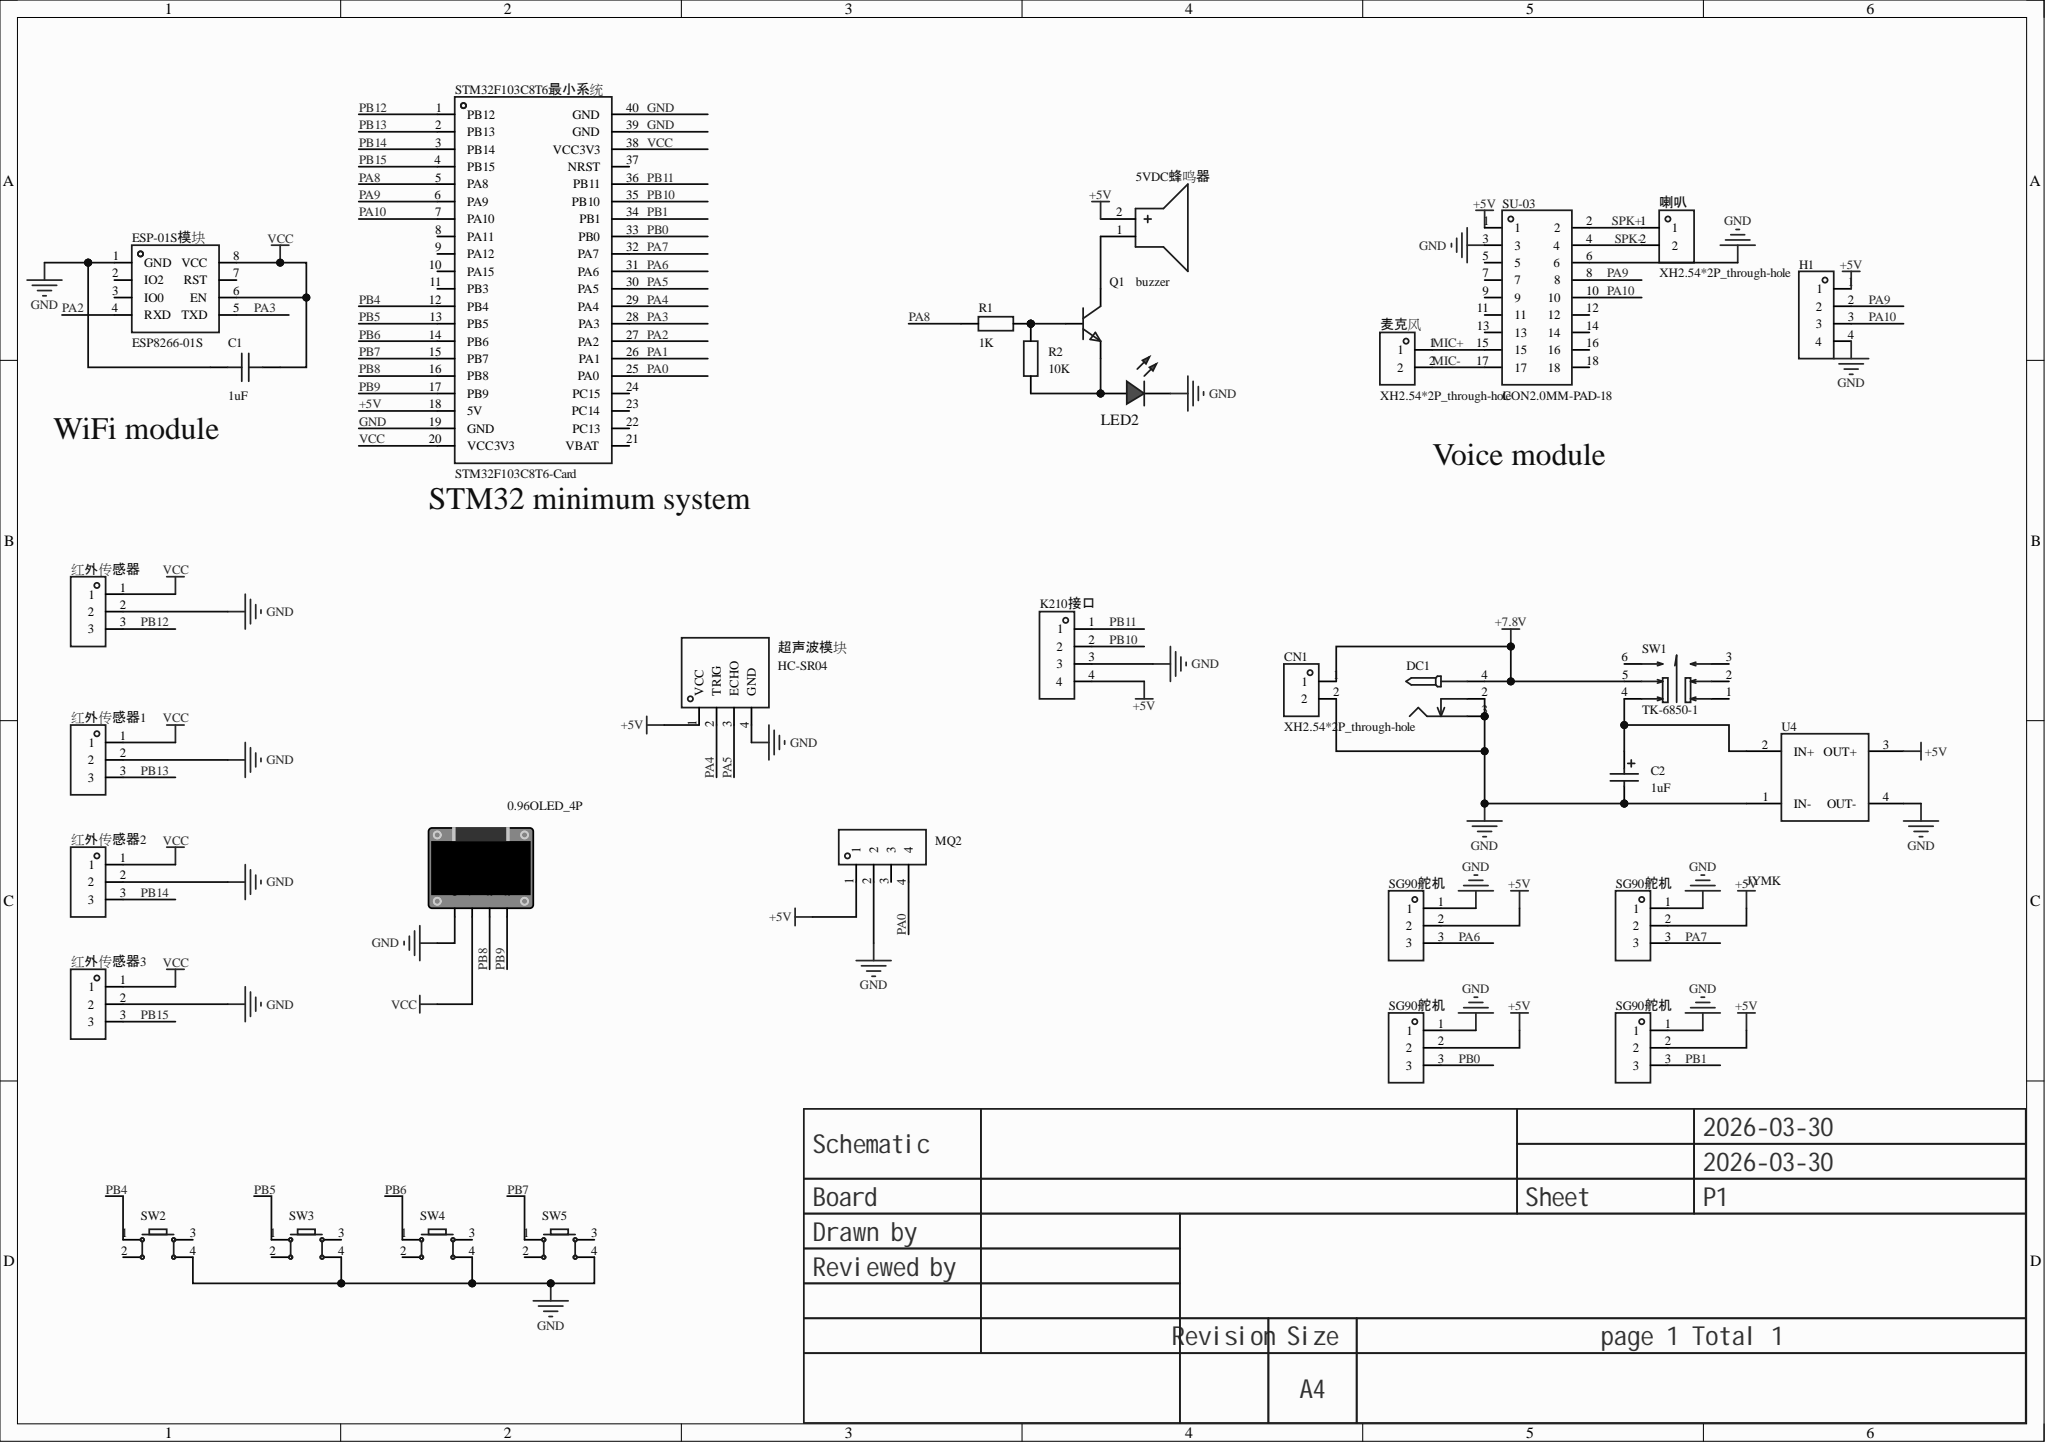Circuit board | Altium Designer | 33 parts | 36 nets
Bill of materials:
Comment,Description,Designator,Footprint,LibRef,Quantity
"","","0.96OLED_4P","0.96OLED_4P","0.96OLED模块_4P","1"
"buzzer","","5VDC蜂鸣器","BUZ-TH_BD12.0-P6.00-D0.9-RD","buzzer","1"
"1uF","","C1","C0603","CAP_0603","1"
"1uF","","C2","C_Ele_SMD_3x5.4mm","C_Ele_SMD_3x5.4mm","1"
"XH2.54*2P_through-hole","","CN1, 喇叭, 麦克风","CONN-TH_2P-P2.50-XH2.54-2P","XH2.54*2P_直插","3"
"","","DC1","DC-2.0","DC-005_2.0","1"
"ESP8266-01S","","ESP-01S模块","WIFIM-TH_ESP8266-01S","ESP8266-01S","1"
"","","H1","HDR-TH_4P-P2.54-V-M","HDR-M_2.54_1x4P","1"
"","","K210接口, MQ2","HDR-TH_4P-P2.54-V-F","HDR-F_2.54_1x4P","2"
"","","LED2","LED_0603","LED_0603-R","1"
"","","Q1","S8050_SOT-23","S8050_SOT_NPN","1"
"1K","","R1","R0603","Res_0603","1"
"10K","","R2","R0603","Res_0603","1"
"","","","HDR-TH_3P-P2.54-V-F","HDR-F_2.54_1x3P","8"
"STM32F103C8T6-Card","","STM32F103C8T6最小系统","CONN-TH_L53.3-W22.9_STM32F103C8T6-CARD","STM32F103C8T6-Card","1"
"CON2.0MM-PAD-18","","SU-03","CONN-TH_18P-P2.00_C9900078766","CON2.0MM-PAD-18","1"
"TK-6850-1","Circuit structure: DPDT; Self-lock/no-lock: self-lock; Mounting type: through-hole; Operating force: 2.4N; Operating life: -;","SW1","SW-TH_TK-6850-1","TK-6850-1","1"
"","","SW2, SW3, SW4, SW5","SW-TH_4P-L6.0-W6.0-P4.50-LS6.5","Key_TH_6x6x6","4"
"","","U4","JYMK","JYMK","1"
"HC-SR04","","超声波模块","TH_HC-SR04V","HC-SR04","1"
Netlist (Protel format):
[
0.96OLED_4P
0.96OLED_4P




]
[
5VDC蜂鸣器
BUZ-TH_BD12.0-P6.00-D0.9-RD
buzzer



]
[
C1
C0603
1uF



]
[
C2
C_Ele_SMD_3x5.4mm
1uF



]
[
CN1
CONN-TH_2P-P2.50-XH2.54-2P
XH2.54*2P_through-hole



]
[
DC1
DC-2.0




]
[
ESP-01S模块
WIFIM-TH_ESP8266-01S
ESP8266-01S



]
[
H1
HDR-TH_4P-P2.54-V-M




]
[
K210接口
HDR-TH_4P-P2.54-V-F




]
[
LED2
LED_0603




]
[
MQ2
HDR-TH_4P-P2.54-V-F




]
[
Q1
S8050_SOT-23




]
[
R1
R0603
1K



]
[
R2
R0603
10K



]
[
SG90舵机
HDR-TH_3P-P2.54-V-F




]
[
SG90舵机
HDR-TH_3P-P2.54-V-F




]
[
SG90舵机
HDR-TH_3P-P2.54-V-F




]
[
SG90舵机
HDR-TH_3P-P2.54-V-F




]
[
STM32F103C8T6最小系统
CONN-TH_L53.3-W22.9_STM32F103C8T6-CARD
STM32F103C8T6-Card



]
[
SU-03
CONN-TH_18P-P2.00_C9900078766
CON2.0MM-PAD-18



]
[
SW1
SW-TH_TK-6850-1
TK-6850-1



]
[
SW2
SW-TH_4P-L6.0-W6.0-P4.50-LS6.5




]
[
SW3
SW-TH_4P-L6.0-W6.0-P4.50-LS6.5




]
[
SW4
SW-TH_4P-L6.0-W6.0-P4.50-LS6.5




]
[
SW5
SW-TH_4P-L6.0-W6.0-P4.50-LS6.5




]
[
U4
JYMK




]
[
喇叭
CONN-TH_2P-P2.50-XH2.54-2P
XH2.54*2P_through-hole



]
[
红外传感器
HDR-TH_3P-P2.54-V-F




]
[
红外传感器1
HDR-TH_3P-P2.54-V-F




]
[
红外传感器2
HDR-TH_3P-P2.54-V-F




]
[
红外传感器3
HDR-TH_3P-P2.54-V-F




]
[
超声波模块
TH_HC-SR04V
HC-SR04



]
[
麦克风
CONN-TH_2P-P2.50-XH2.54-2P
XH2.54*2P_through-hole



]
(
VCC
0.96OLED_4P-2
C1-2
ESP-01S模块-6
ESP-01S模块-8
STM32F103C8T6最小系统-20
STM32F103C8T6最小系统-38
红外传感器-1
红外传感器1-1
红外传感器2-1
红外传感器3-1
)
(
SPK-
SU-03-4
喇叭-2
)
(
SPK+
SU-03-2
喇叭-1
)
(
PB15
STM32F103C8T6最小系统-4
红外传感器3-3
)
(
PB14
STM32F103C8T6最小系统-3
红外传感器2-3
)
(
PB13
STM32F103C8T6最小系统-2
红外传感器1-3
)
(
PB12
STM32F103C8T6最小系统-1
红外传感器-3
)
(
PB11
K210接口-1
STM32F103C8T6最小系统-36
)
(
PB10
K210接口-2
STM32F103C8T6最小系统-35
)
(
PB9
0.96OLED_4P-4
STM32F103C8T6最小系统-17
)
(
PB8
0.96OLED_4P-3
STM32F103C8T6最小系统-16
)
(
PB7
STM32F103C8T6最小系统-15
SW5-1
)
(
PB6
STM32F103C8T6最小系统-14
SW4-1
)
(
PB5
STM32F103C8T6最小系统-13
SW3-1
)
(
PB4
STM32F103C8T6最小系统-12
SW2-1
)
(
PB1
SG90舵机-3
STM32F103C8T6最小系统-34
)
(
PB0
SG90舵机-3
STM32F103C8T6最小系统-33
)
(
PA10
H1-3
STM32F103C8T6最小系统-7
SU-03-10
)
(
PA9
H1-2
STM32F103C8T6最小系统-6
SU-03-8
)
(
PA8
R1-1
STM32F103C8T6最小系统-5
)
(
PA7
SG90舵机-3
STM32F103C8T6最小系统-32
)
(
PA6
SG90舵机-3
STM32F103C8T6最小系统-31
)
(
PA5
STM32F103C8T6最小系统-30
超声波模块-3
)
(
PA4
STM32F103C8T6最小系统-29
超声波模块-2
)
(
PA3
ESP-01S模块-5
STM32F103C8T6最小系统-28
)
(
PA2
ESP-01S模块-4
STM32F103C8T6最小系统-27
)
(
PA0
MQ2-4
STM32F103C8T6最小系统-25
)
(
NetQ1_1
Q1-1
R1-2
R2-2
)
(
NetLED2_2
LED2-2
Q1-2
R2-1
)
(
NetC2_1
C2-1
SW1-4
U4-2
)
(
Net5VDC蜂鸣器_1
5VDC蜂鸣器-1
Q1-3
)
(
MIC-
SU-03-17
麦克风-2
)
(
MIC+
SU-03-15
麦克风-1
)
(
GND
0.96OLED_4P-1
C1-1
C2-2
CN1-2
DC1-2
DC1-3
ESP-01S模块-1
H1-4
K210接口-3
LED2-1
MQ2-2
SG90舵机-1
SG90舵机-1
SG90舵机-1
SG90舵机-1
STM32F103C8T6最小系统-19
STM32F103C8T6最小系统-39
STM32F103C8T6最小系统-40
SU-03-3
SU-03-6
SW2-4
SW3-4
SW4-4
SW5-4
U4-1
U4-4
红外传感器-2
红外传感器1-2
红外传感器2-2
红外传感器3-2
超声波模块-4
)
(
+7.8V
CN1-1
DC1-4
SW1-5
)
(
+5V
5VDC蜂鸣器-2
H1-1
K210接口-4
MQ2-1
SG90舵机-2
SG90舵机-2
SG90舵机-2
SG90舵机-2
STM32F103C8T6最小系统-18
SU-03-1
U4-3
超声波模块-1
)